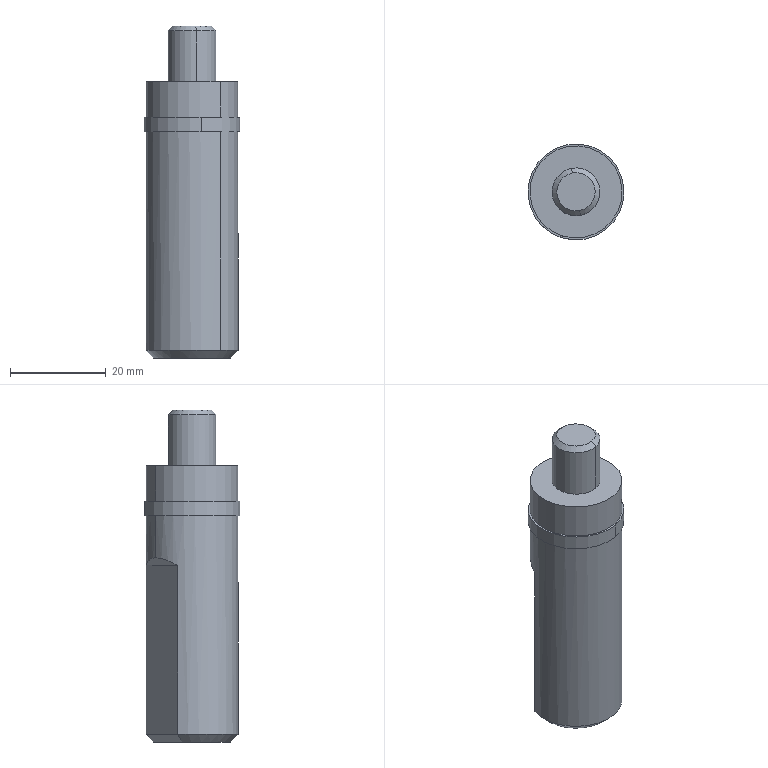Part | SolidWorks | features BaseBody 1 | 1 solid | 19 faces | box 20 x 20 x 69.2 mm | volume 17144 mm3 | cylinder 8 | plane 8 | cone 3 | commonest cylinder face diameters 19.2 x4 10 x2 20 x2
STEP:
#1=CARTESIAN_POINT('',(-577.044,-13.249,-437.6));
#2=VERTEX_POINT('',#1);
#3=CARTESIAN_POINT('',(-578.93,-3.429,-437.6));
#4=VERTEX_POINT('',#3);
#5=CARTESIAN_POINT('',(-577.987,-8.339,-437.6));
#6=DIRECTION('',(0.,0.,1.));
#7=DIRECTION('',(-1.,0.,0.));
#8=AXIS2_PLACEMENT_3D('',#5,#6,#7);
#9=CIRCLE('',#8,5.);
#10=EDGE_CURVE('',#2,#4,#9,.T.);
#11=ORIENTED_EDGE('',*,*,#10,.T.);
#12=CARTESIAN_POINT('',(-578.93,-3.429,-427.));
#13=VERTEX_POINT('',#12);
#14=CARTESIAN_POINT('',(-578.93,-3.429,-445.));
#15=DIRECTION('',(0.,0.,1.));
#16=VECTOR('',#15,1000.);
#17=LINE('',#14,#16);
#18=EDGE_CURVE('',#4,#13,#17,.T.);
#19=ORIENTED_EDGE('',*,*,#18,.T.);
#20=CARTESIAN_POINT('',(-577.044,-13.249,-427.));
#21=VERTEX_POINT('',#20);
#22=CARTESIAN_POINT('',(-577.987,-8.339,-427.));
#23=DIRECTION('',(0.,0.,-1.));
#24=DIRECTION('',(0.1886,-0.982,0.));
#25=AXIS2_PLACEMENT_3D('',#22,#23,#24);
#26=CIRCLE('',#25,5.);
#27=EDGE_CURVE('',#13,#21,#26,.T.);
#28=ORIENTED_EDGE('',*,*,#27,.T.);
#29=CARTESIAN_POINT('',(-577.044,-13.249,-445.));
#30=DIRECTION('',(0.,0.,1.));
#31=VECTOR('',#30,1000.);
#32=LINE('',#29,#31);
#33=EDGE_CURVE('',#2,#21,#32,.T.);
#34=ORIENTED_EDGE('',*,*,#33,.F.);
#35=EDGE_LOOP('',(#11,#19,#28,#34));
#36=FACE_OUTER_BOUND('',#35,.T.);
#37=CARTESIAN_POINT('',(-577.987,-8.339,-445.));
#38=DIRECTION('',(0.,0.,1.));
#39=DIRECTION('',(0.1886,-0.982,0.));
#40=AXIS2_PLACEMENT_3D('',#37,#38,#39);
#41=CYLINDRICAL_SURFACE('',#40,5.);
#42=ADVANCED_FACE('',(#36),#41,.T.);
#43=CARTESIAN_POINT('',(-577.232,-12.267,-426.));
#44=VERTEX_POINT('',#43);
#45=CARTESIAN_POINT('',(-578.741,-4.411,-426.));
#46=VERTEX_POINT('',#45);
#47=CARTESIAN_POINT('',(-577.987,-8.339,-426.));
#48=DIRECTION('',(0.,0.,1.));
#49=DIRECTION('',(0.1886,-0.982,0.));
#50=AXIS2_PLACEMENT_3D('',#47,#48,#49);
#51=CIRCLE('',#50,4.);
#52=EDGE_CURVE('',#44,#46,#51,.T.);
#53=ORIENTED_EDGE('',*,*,#52,.F.);
#54=CARTESIAN_POINT('',(-577.232,-12.267,-426.));
#55=DIRECTION('',(0.1334,-0.6944,-0.7071));
#56=VECTOR('',#55,1000.);
#57=LINE('',#54,#56);
#58=EDGE_CURVE('',#44,#21,#57,.T.);
#59=ORIENTED_EDGE('',*,*,#58,.T.);
#60=ORIENTED_EDGE('',*,*,#27,.F.);
#61=CARTESIAN_POINT('',(-578.741,-4.411,-426.));
#62=DIRECTION('',(-0.1334,0.6944,-0.7071));
#63=VECTOR('',#62,1000.);
#64=LINE('',#61,#63);
#65=EDGE_CURVE('',#46,#13,#64,.T.);
#66=ORIENTED_EDGE('',*,*,#65,.F.);
#67=EDGE_LOOP('',(#53,#59,#60,#66));
#68=FACE_OUTER_BOUND('',#67,.T.);
#69=CARTESIAN_POINT('',(-577.987,-8.339,-426.));
#70=DIRECTION('',(0.,0.,-1.));
#71=DIRECTION('',(-0.1886,0.982,0.));
#72=AXIS2_PLACEMENT_3D('',#69,#70,#71);
#73=CONICAL_SURFACE('',#72,4.,0.7854);
#74=ADVANCED_FACE('',(#68),#73,.T.);
#75=CARTESIAN_POINT('',(-572.04,-15.875,-445.));
#76=VERTEX_POINT('',#75);
#77=CARTESIAN_POINT('',(-583.933,-0.8028,-445.));
#78=VERTEX_POINT('',#77);
#79=CARTESIAN_POINT('',(-577.987,-8.339,-445.));
#80=DIRECTION('',(0.,0.,-1.));
#81=DIRECTION('',(1.,0.,0.));
#82=AXIS2_PLACEMENT_3D('',#79,#80,#81);
#83=CIRCLE('',#82,9.6);
#84=EDGE_CURVE('',#76,#78,#83,.T.);
#85=ORIENTED_EDGE('',*,*,#84,.F.);
#86=CARTESIAN_POINT('',(-572.04,-15.875,-437.6));
#87=VERTEX_POINT('',#86);
#88=CARTESIAN_POINT('',(-572.04,-15.875,-437.6));
#89=DIRECTION('',(0.,0.,1.));
#90=VECTOR('',#89,1000.);
#91=LINE('',#88,#90);
#92=EDGE_CURVE('',#76,#87,#91,.T.);
#93=ORIENTED_EDGE('',*,*,#92,.T.);
#94=CARTESIAN_POINT('',(-583.933,-0.8028,-437.6));
#95=VERTEX_POINT('',#94);
#96=CARTESIAN_POINT('',(-577.987,-8.339,-437.6));
#97=DIRECTION('',(0.,0.,1.));
#98=DIRECTION('',(0.6195,-0.785,0.));
#99=AXIS2_PLACEMENT_3D('',#96,#97,#98);
#100=CIRCLE('',#99,9.6);
#101=EDGE_CURVE('',#95,#87,#100,.T.);
#102=ORIENTED_EDGE('',*,*,#101,.F.);
#103=CARTESIAN_POINT('',(-583.933,-0.8028,-437.6));
#104=DIRECTION('',(0.,0.,1.));
#105=VECTOR('',#104,1000.);
#106=LINE('',#103,#105);
#107=EDGE_CURVE('',#78,#95,#106,.T.);
#108=ORIENTED_EDGE('',*,*,#107,.F.);
#109=EDGE_LOOP('',(#85,#93,#102,#108));
#110=FACE_OUTER_BOUND('',#109,.T.);
#111=CARTESIAN_POINT('',(-577.987,-8.339,-437.6));
#112=DIRECTION('',(0.,0.,1.));
#113=DIRECTION('',(-0.6195,0.785,0.));
#114=AXIS2_PLACEMENT_3D('',#111,#112,#113);
#115=CYLINDRICAL_SURFACE('',#114,9.6);
#116=ADVANCED_FACE('',(#110),#115,.T.);
#117=CARTESIAN_POINT('',(-579.873,1.481,-448.));
#118=VERTEX_POINT('',#117);
#119=CARTESIAN_POINT('',(-576.1,-18.16,-448.));
#120=VERTEX_POINT('',#119);
#121=CARTESIAN_POINT('',(-577.987,-8.339,-448.));
#122=DIRECTION('',(0.,0.,-1.));
#123=DIRECTION('',(-0.1886,0.982,0.));
#124=AXIS2_PLACEMENT_3D('',#121,#122,#123);
#125=CIRCLE('',#124,10.);
#126=EDGE_CURVE('',#118,#120,#125,.T.);
#127=ORIENTED_EDGE('',*,*,#126,.F.);
#128=CARTESIAN_POINT('',(-579.873,1.481,-445.));
#129=VERTEX_POINT('',#128);
#130=CARTESIAN_POINT('',(-579.873,1.481,-448.));
#131=DIRECTION('',(0.,0.,1.));
#132=VECTOR('',#131,1000.);
#133=LINE('',#130,#132);
#134=EDGE_CURVE('',#118,#129,#133,.T.);
#135=ORIENTED_EDGE('',*,*,#134,.T.);
#136=CARTESIAN_POINT('',(-576.1,-18.16,-445.));
#137=VERTEX_POINT('',#136);
#138=CARTESIAN_POINT('',(-577.987,-8.339,-445.));
#139=DIRECTION('',(0.,0.,-1.));
#140=DIRECTION('',(-0.1886,0.982,0.));
#141=AXIS2_PLACEMENT_3D('',#138,#139,#140);
#142=CIRCLE('',#141,10.);
#143=EDGE_CURVE('',#129,#137,#142,.T.);
#144=ORIENTED_EDGE('',*,*,#143,.T.);
#145=CARTESIAN_POINT('',(-576.1,-18.16,-448.));
#146=DIRECTION('',(0.,0.,1.));
#147=VECTOR('',#146,1000.);
#148=LINE('',#145,#147);
#149=EDGE_CURVE('',#120,#137,#148,.T.);
#150=ORIENTED_EDGE('',*,*,#149,.F.);
#151=EDGE_LOOP('',(#127,#135,#144,#150));
#152=FACE_OUTER_BOUND('',#151,.T.);
#153=CARTESIAN_POINT('',(-577.987,-8.339,-448.));
#154=DIRECTION('',(0.,0.,1.));
#155=DIRECTION('',(0.1886,-0.982,0.));
#156=AXIS2_PLACEMENT_3D('',#153,#154,#155);
#157=CYLINDRICAL_SURFACE('',#156,10.);
#158=ADVANCED_FACE('',(#152),#157,.T.);
#159=CARTESIAN_POINT('',(-587.108,-5.346,-493.6));
#160=VERTEX_POINT('',#159);
#161=CARTESIAN_POINT('',(-572.04,-15.875,-493.6));
#162=VERTEX_POINT('',#161);
#163=CARTESIAN_POINT('',(-577.987,-8.339,-493.6));
#164=DIRECTION('',(0.,0.,1.));
#165=DIRECTION('',(0.6195,-0.785,0.));
#166=AXIS2_PLACEMENT_3D('',#163,#164,#165);
#167=CIRCLE('',#166,9.6);
#168=EDGE_CURVE('',#160,#162,#167,.T.);
#169=ORIENTED_EDGE('',*,*,#168,.T.);
#170=CARTESIAN_POINT('',(-572.04,-15.875,-448.));
#171=VERTEX_POINT('',#170);
#172=CARTESIAN_POINT('',(-572.04,-15.875,-437.6));
#173=DIRECTION('',(0.,0.,1.));
#174=VECTOR('',#173,1000.);
#175=LINE('',#172,#174);
#176=EDGE_CURVE('',#162,#171,#175,.T.);
#177=ORIENTED_EDGE('',*,*,#176,.T.);
#178=CARTESIAN_POINT('',(-583.933,-0.8028,-448.));
#179=VERTEX_POINT('',#178);
#180=CARTESIAN_POINT('',(-577.987,-8.339,-448.));
#181=DIRECTION('',(0.,0.,-1.));
#182=DIRECTION('',(1.,0.,0.));
#183=AXIS2_PLACEMENT_3D('',#180,#181,#182);
#184=CIRCLE('',#183,9.6);
#185=EDGE_CURVE('',#171,#179,#184,.T.);
#186=ORIENTED_EDGE('',*,*,#185,.T.);
#187=CARTESIAN_POINT('',(-583.933,-0.8028,-456.8));
#188=VERTEX_POINT('',#187);
#189=CARTESIAN_POINT('',(-583.933,-0.8028,-437.6));
#190=DIRECTION('',(0.,0.,1.));
#191=VECTOR('',#190,1000.);
#192=LINE('',#189,#191);
#193=EDGE_CURVE('',#188,#179,#192,.T.);
#194=ORIENTED_EDGE('',*,*,#193,.F.);
#195=CARTESIAN_POINT('',(-587.108,-5.346,-458.4));
#196=VERTEX_POINT('',#195);
#197=CARTESIAN_POINT('',(-583.933,-0.8028,-456.8));
#198=CARTESIAN_POINT('',(-585.426,-1.981,-456.8));
#199=CARTESIAN_POINT('',(-586.515,-3.539,-457.349));
#200=CARTESIAN_POINT('',(-587.108,-5.346,-458.4));
#201=(BOUNDED_CURVE()B_SPLINE_CURVE(3,(#197,#198,#199,#200),.UNSPECIFIED.,.F.,.F.)B_SPLINE_CURVE_WITH_KNOTS((4,4),(0.,0.5857),.UNSPECIFIED.)CURVE()GEOMETRIC_REPRESENTATION_ITEM()RATIONAL_B_SPLINE_CURVE((1.,0.9716,0.9716,1.))REPRESENTATION_ITEM(''));
#202=EDGE_CURVE('',#188,#196,#201,.T.);
#203=ORIENTED_EDGE('',*,*,#202,.T.);
#204=CARTESIAN_POINT('',(-587.108,-5.346,-456.8));
#205=DIRECTION('',(0.,0.,1.));
#206=VECTOR('',#205,1000.);
#207=LINE('',#204,#206);
#208=EDGE_CURVE('',#160,#196,#207,.T.);
#209=ORIENTED_EDGE('',*,*,#208,.F.);
#210=EDGE_LOOP('',(#169,#177,#186,#194,#203,#209));
#211=FACE_OUTER_BOUND('',#210,.T.);
#212=CARTESIAN_POINT('',(-577.987,-8.339,-437.6));
#213=DIRECTION('',(0.,0.,1.));
#214=DIRECTION('',(-0.6195,0.785,0.));
#215=AXIS2_PLACEMENT_3D('',#212,#213,#214);
#216=CYLINDRICAL_SURFACE('',#215,9.6);
#217=ADVANCED_FACE('',(#211),#216,.T.);
#218=ORIENTED_EDGE('',*,*,#176,.F.);
#219=CARTESIAN_POINT('',(-578.777,1.228,-493.6));
#220=VERTEX_POINT('',#219);
#221=CARTESIAN_POINT('',(-577.987,-8.339,-493.6));
#222=DIRECTION('',(0.,0.,1.));
#223=DIRECTION('',(0.6195,-0.785,0.));
#224=AXIS2_PLACEMENT_3D('',#221,#222,#223);
#225=CIRCLE('',#224,9.6);
#226=EDGE_CURVE('',#162,#220,#225,.T.);
#227=ORIENTED_EDGE('',*,*,#226,.T.);
#228=CARTESIAN_POINT('',(-578.777,1.228,-458.4));
#229=VERTEX_POINT('',#228);
#230=CARTESIAN_POINT('',(-578.777,1.228,-456.8));
#231=DIRECTION('',(0.,0.,1.));
#232=VECTOR('',#231,1000.);
#233=LINE('',#230,#232);
#234=EDGE_CURVE('',#220,#229,#233,.T.);
#235=ORIENTED_EDGE('',*,*,#234,.T.);
#236=CARTESIAN_POINT('',(-578.777,1.228,-458.4));
#237=CARTESIAN_POINT('',(-580.672,1.072,-457.349));
#238=CARTESIAN_POINT('',(-582.441,0.3751,-456.8));
#239=CARTESIAN_POINT('',(-583.933,-0.8028,-456.8));
#240=(BOUNDED_CURVE()B_SPLINE_CURVE(3,(#236,#237,#238,#239),.UNSPECIFIED.,.F.,.F.)B_SPLINE_CURVE_WITH_KNOTS((4,4),(5.697,6.283),.UNSPECIFIED.)CURVE()GEOMETRIC_REPRESENTATION_ITEM()RATIONAL_B_SPLINE_CURVE((1.,0.9716,0.9716,1.))REPRESENTATION_ITEM(''));
#241=EDGE_CURVE('',#229,#188,#240,.T.);
#242=ORIENTED_EDGE('',*,*,#241,.T.);
#243=ORIENTED_EDGE('',*,*,#193,.T.);
#244=CARTESIAN_POINT('',(-577.987,-8.339,-448.));
#245=DIRECTION('',(0.,0.,-1.));
#246=DIRECTION('',(1.,0.,0.));
#247=AXIS2_PLACEMENT_3D('',#244,#245,#246);
#248=CIRCLE('',#247,9.6);
#249=EDGE_CURVE('',#179,#171,#248,.T.);
#250=ORIENTED_EDGE('',*,*,#249,.T.);
#251=EDGE_LOOP('',(#218,#227,#235,#242,#243,#250));
#252=FACE_OUTER_BOUND('',#251,.T.);
#253=CARTESIAN_POINT('',(-577.987,-8.339,-437.6));
#254=DIRECTION('',(0.,0.,1.));
#255=DIRECTION('',(-0.6195,0.785,0.));
#256=AXIS2_PLACEMENT_3D('',#253,#254,#255);
#257=CYLINDRICAL_SURFACE('',#256,9.6);
#258=ADVANCED_FACE('',(#252),#257,.T.);
#259=CARTESIAN_POINT('',(-585.719,-6.288,-495.2));
#260=VERTEX_POINT('',#259);
#261=CARTESIAN_POINT('',(-578.183,-0.3415,-495.2));
#262=VERTEX_POINT('',#261);
#263=CARTESIAN_POINT('',(-586.117,-6.602,-495.2));
#264=DIRECTION('',(0.785,0.6195,0.));
#265=VECTOR('',#264,1000.);
#266=LINE('',#263,#265);
#267=EDGE_CURVE('',#260,#262,#266,.T.);
#268=ORIENTED_EDGE('',*,*,#267,.T.);
#269=CARTESIAN_POINT('',(-577.987,-8.339,-495.2));
#270=DIRECTION('',(0.,0.,-1.));
#271=DIRECTION('',(0.6195,-0.785,0.));
#272=AXIS2_PLACEMENT_3D('',#269,#270,#271);
#273=CIRCLE('',#272,8.);
#274=EDGE_CURVE('',#262,#260,#273,.T.);
#275=ORIENTED_EDGE('',*,*,#274,.T.);
#276=EDGE_LOOP('',(#268,#275));
#277=FACE_OUTER_BOUND('',#276,.T.);
#278=CARTESIAN_POINT('',(-577.987,-8.339,-495.2));
#279=DIRECTION('',(0.,0.,-1.));
#280=DIRECTION('',(0.6195,-0.785,0.));
#281=AXIS2_PLACEMENT_3D('',#278,#279,#280);
#282=PLANE('',#281);
#283=ADVANCED_FACE('',(#277),#282,.T.);
#284=ORIENTED_EDGE('',*,*,#208,.T.);
#285=CARTESIAN_POINT('',(-587.108,-5.346,-458.4));
#286=DIRECTION('',(0.785,0.6195,0.));
#287=VECTOR('',#286,1000.);
#288=LINE('',#285,#287);
#289=EDGE_CURVE('',#196,#229,#288,.T.);
#290=ORIENTED_EDGE('',*,*,#289,.T.);
#291=ORIENTED_EDGE('',*,*,#234,.F.);
#292=CARTESIAN_POINT('',(-578.777,1.228,-493.6));
#293=DIRECTION('',(-0.785,-0.6195,0.));
#294=VECTOR('',#293,1000.);
#295=LINE('',#292,#294);
#296=EDGE_CURVE('',#220,#160,#295,.T.);
#297=ORIENTED_EDGE('',*,*,#296,.T.);
#298=EDGE_LOOP('',(#284,#290,#291,#297));
#299=FACE_OUTER_BOUND('',#298,.T.);
#300=CARTESIAN_POINT('',(-587.108,-5.346,-456.8));
#301=DIRECTION('',(0.6195,-0.785,0.));
#302=DIRECTION('',(0.785,0.6195,0.));
#303=AXIS2_PLACEMENT_3D('',#300,#301,#302);
#304=PLANE('',#303);
#305=ADVANCED_FACE('',(#299),#304,.F.);
#306=CARTESIAN_POINT('',(-578.183,-0.3415,-495.2));
#307=CARTESIAN_POINT('',(-578.373,0.186,-494.668));
#308=CARTESIAN_POINT('',(-578.572,0.7089,-494.135));
#309=CARTESIAN_POINT('',(-578.777,1.228,-493.6));
#310=B_SPLINE_CURVE_WITH_KNOTS('',3,(#306,#307,#308,#309),.UNSPECIFIED.,.F.,.F.,(4,4),(0.,0.002319),.UNSPECIFIED.);
#311=EDGE_CURVE('',#262,#220,#310,.T.);
#312=ORIENTED_EDGE('',*,*,#311,.F.);
#313=ORIENTED_EDGE('',*,*,#267,.F.);
#314=CARTESIAN_POINT('',(-587.108,-5.346,-493.6));
#315=CARTESIAN_POINT('',(-586.651,-5.666,-494.135));
#316=CARTESIAN_POINT('',(-586.188,-5.98,-494.668));
#317=CARTESIAN_POINT('',(-585.719,-6.288,-495.2));
#318=B_SPLINE_CURVE_WITH_KNOTS('',3,(#314,#315,#316,#317),.UNSPECIFIED.,.F.,.F.,(4,4),(0.,0.002319),.UNSPECIFIED.);
#319=EDGE_CURVE('',#160,#260,#318,.T.);
#320=ORIENTED_EDGE('',*,*,#319,.F.);
#321=ORIENTED_EDGE('',*,*,#296,.F.);
#322=EDGE_LOOP('',(#312,#313,#320,#321));
#323=FACE_OUTER_BOUND('',#322,.T.);
#324=CARTESIAN_POINT('',(-587.108,-5.346,-493.6));
#325=DIRECTION('',(-0.438,0.5551,-0.7071));
#326=DIRECTION('',(-0.785,-0.6195,0.));
#327=AXIS2_PLACEMENT_3D('',#324,#325,#326);
#328=PLANE('',#327);
#329=ADVANCED_FACE('',(#323),#328,.T.);
#330=ORIENTED_EDGE('',*,*,#319,.T.);
#331=ORIENTED_EDGE('',*,*,#274,.F.);
#332=ORIENTED_EDGE('',*,*,#311,.T.);
#333=ORIENTED_EDGE('',*,*,#226,.F.);
#334=ORIENTED_EDGE('',*,*,#168,.F.);
#335=EDGE_LOOP('',(#330,#331,#332,#333,#334));
#336=FACE_OUTER_BOUND('',#335,.T.);
#337=CARTESIAN_POINT('',(-577.987,-8.339,-495.2));
#338=DIRECTION('',(0.,0.,1.));
#339=DIRECTION('',(-0.6195,0.785,0.));
#340=AXIS2_PLACEMENT_3D('',#337,#338,#339);
#341=CONICAL_SURFACE('',#340,8.,0.7854);
#342=ADVANCED_FACE('',(#336),#341,.T.);
#343=ORIENTED_EDGE('',*,*,#289,.F.);
#344=ORIENTED_EDGE('',*,*,#202,.F.);
#345=ORIENTED_EDGE('',*,*,#241,.F.);
#346=EDGE_LOOP('',(#343,#344,#345));
#347=FACE_OUTER_BOUND('',#346,.T.);
#348=CARTESIAN_POINT('',(-583.933,-0.8028,-456.8));
#349=DIRECTION('',(0.438,-0.5551,0.7071));
#350=DIRECTION('',(0.785,0.6195,0.));
#351=AXIS2_PLACEMENT_3D('',#348,#349,#350);
#352=PLANE('',#351);
#353=ADVANCED_FACE('',(#347),#352,.F.);
#354=CARTESIAN_POINT('',(-577.987,-8.339,-448.));
#355=DIRECTION('',(0.,0.,-1.));
#356=DIRECTION('',(-0.1886,0.982,0.));
#357=AXIS2_PLACEMENT_3D('',#354,#355,#356);
#358=CIRCLE('',#357,10.);
#359=EDGE_CURVE('',#120,#118,#358,.T.);
#360=ORIENTED_EDGE('',*,*,#359,.T.);
#361=ORIENTED_EDGE('',*,*,#126,.T.);
#362=EDGE_LOOP('',(#360,#361));
#363=FACE_OUTER_BOUND('',#362,.T.);
#364=ORIENTED_EDGE('',*,*,#249,.F.);
#365=ORIENTED_EDGE('',*,*,#185,.F.);
#366=EDGE_LOOP('',(#364,#365));
#367=FACE_BOUND('',#366,.T.);
#368=CARTESIAN_POINT('',(-577.987,-8.339,-448.));
#369=DIRECTION('',(0.,0.,-1.));
#370=DIRECTION('',(-0.1886,0.982,0.));
#371=AXIS2_PLACEMENT_3D('',#368,#369,#370);
#372=PLANE('',#371);
#373=ADVANCED_FACE('',(#363,#367),#372,.T.);
#374=CARTESIAN_POINT('',(-577.987,-8.339,-445.));
#375=DIRECTION('',(0.,0.,-1.));
#376=DIRECTION('',(-0.1886,0.982,0.));
#377=AXIS2_PLACEMENT_3D('',#374,#375,#376);
#378=CIRCLE('',#377,10.);
#379=EDGE_CURVE('',#137,#129,#378,.T.);
#380=ORIENTED_EDGE('',*,*,#379,.F.);
#381=ORIENTED_EDGE('',*,*,#143,.F.);
#382=EDGE_LOOP('',(#380,#381));
#383=FACE_OUTER_BOUND('',#382,.T.);
#384=CARTESIAN_POINT('',(-577.987,-8.339,-445.));
#385=DIRECTION('',(0.,0.,-1.));
#386=DIRECTION('',(1.,0.,0.));
#387=AXIS2_PLACEMENT_3D('',#384,#385,#386);
#388=CIRCLE('',#387,9.6);
#389=EDGE_CURVE('',#78,#76,#388,.T.);
#390=ORIENTED_EDGE('',*,*,#389,.T.);
#391=ORIENTED_EDGE('',*,*,#84,.T.);
#392=EDGE_LOOP('',(#390,#391));
#393=FACE_BOUND('',#392,.T.);
#394=CARTESIAN_POINT('',(-577.987,-8.339,-445.));
#395=DIRECTION('',(0.,0.,-1.));
#396=DIRECTION('',(-0.1886,0.982,0.));
#397=AXIS2_PLACEMENT_3D('',#394,#395,#396);
#398=PLANE('',#397);
#399=ADVANCED_FACE('',(#383,#393),#398,.F.);
#400=ORIENTED_EDGE('',*,*,#134,.F.);
#401=ORIENTED_EDGE('',*,*,#359,.F.);
#402=ORIENTED_EDGE('',*,*,#149,.T.);
#403=ORIENTED_EDGE('',*,*,#379,.T.);
#404=EDGE_LOOP('',(#400,#401,#402,#403));
#405=FACE_OUTER_BOUND('',#404,.T.);
#406=CARTESIAN_POINT('',(-577.987,-8.339,-448.));
#407=DIRECTION('',(0.,0.,1.));
#408=DIRECTION('',(0.1886,-0.982,0.));
#409=AXIS2_PLACEMENT_3D('',#406,#407,#408);
#410=CYLINDRICAL_SURFACE('',#409,10.);
#411=ADVANCED_FACE('',(#405),#410,.T.);
#412=ORIENTED_EDGE('',*,*,#10,.F.);
#413=CARTESIAN_POINT('',(-577.987,-8.339,-437.6));
#414=DIRECTION('',(0.,0.,1.));
#415=DIRECTION('',(-1.,0.,0.));
#416=AXIS2_PLACEMENT_3D('',#413,#414,#415);
#417=CIRCLE('',#416,5.);
#418=EDGE_CURVE('',#4,#2,#417,.T.);
#419=ORIENTED_EDGE('',*,*,#418,.F.);
#420=EDGE_LOOP('',(#412,#419));
#421=FACE_BOUND('',#420,.T.);
#422=ORIENTED_EDGE('',*,*,#101,.T.);
#423=CARTESIAN_POINT('',(-577.987,-8.339,-437.6));
#424=DIRECTION('',(0.,0.,1.));
#425=DIRECTION('',(0.6195,-0.785,0.));
#426=AXIS2_PLACEMENT_3D('',#423,#424,#425);
#427=CIRCLE('',#426,9.6);
#428=EDGE_CURVE('',#87,#95,#427,.T.);
#429=ORIENTED_EDGE('',*,*,#428,.T.);
#430=EDGE_LOOP('',(#422,#429));
#431=FACE_OUTER_BOUND('',#430,.T.);
#432=CARTESIAN_POINT('',(-584.663,0.1218,-437.6));
#433=DIRECTION('',(0.,0.,1.));
#434=DIRECTION('',(-1.,0.,0.));
#435=AXIS2_PLACEMENT_3D('',#432,#433,#434);
#436=PLANE('',#435);
#437=ADVANCED_FACE('',(#421,#431),#436,.T.);
#438=ORIENTED_EDGE('',*,*,#92,.F.);
#439=ORIENTED_EDGE('',*,*,#389,.F.);
#440=ORIENTED_EDGE('',*,*,#107,.T.);
#441=ORIENTED_EDGE('',*,*,#428,.F.);
#442=EDGE_LOOP('',(#438,#439,#440,#441));
#443=FACE_OUTER_BOUND('',#442,.T.);
#444=CARTESIAN_POINT('',(-577.987,-8.339,-437.6));
#445=DIRECTION('',(0.,0.,1.));
#446=DIRECTION('',(-0.6195,0.785,0.));
#447=AXIS2_PLACEMENT_3D('',#444,#445,#446);
#448=CYLINDRICAL_SURFACE('',#447,9.6);
#449=ADVANCED_FACE('',(#443),#448,.T.);
#450=CARTESIAN_POINT('',(-577.987,-8.339,-426.));
#451=DIRECTION('',(0.,0.,1.));
#452=DIRECTION('',(0.1886,-0.982,0.));
#453=AXIS2_PLACEMENT_3D('',#450,#451,#452);
#454=CIRCLE('',#453,4.);
#455=EDGE_CURVE('',#46,#44,#454,.T.);
#456=ORIENTED_EDGE('',*,*,#455,.T.);
#457=ORIENTED_EDGE('',*,*,#52,.T.);
#458=EDGE_LOOP('',(#456,#457));
#459=FACE_OUTER_BOUND('',#458,.T.);
#460=CARTESIAN_POINT('',(-577.987,-8.339,-426.));
#461=DIRECTION('',(0.,0.,1.));
#462=DIRECTION('',(0.1886,-0.982,0.));
#463=AXIS2_PLACEMENT_3D('',#460,#461,#462);
#464=PLANE('',#463);
#465=ADVANCED_FACE('',(#459),#464,.T.);
#466=ORIENTED_EDGE('',*,*,#58,.F.);
#467=ORIENTED_EDGE('',*,*,#455,.F.);
#468=ORIENTED_EDGE('',*,*,#65,.T.);
#469=CARTESIAN_POINT('',(-577.987,-8.339,-427.));
#470=DIRECTION('',(0.,0.,-1.));
#471=DIRECTION('',(0.1886,-0.982,0.));
#472=AXIS2_PLACEMENT_3D('',#469,#470,#471);
#473=CIRCLE('',#472,5.);
#474=EDGE_CURVE('',#21,#13,#473,.T.);
#475=ORIENTED_EDGE('',*,*,#474,.F.);
#476=EDGE_LOOP('',(#466,#467,#468,#475));
#477=FACE_OUTER_BOUND('',#476,.T.);
#478=CARTESIAN_POINT('',(-577.987,-8.339,-426.));
#479=DIRECTION('',(0.,0.,-1.));
#480=DIRECTION('',(-0.1886,0.982,0.));
#481=AXIS2_PLACEMENT_3D('',#478,#479,#480);
#482=CONICAL_SURFACE('',#481,4.,0.7854);
#483=ADVANCED_FACE('',(#477),#482,.T.);
#484=ORIENTED_EDGE('',*,*,#18,.F.);
#485=ORIENTED_EDGE('',*,*,#418,.T.);
#486=ORIENTED_EDGE('',*,*,#33,.T.);
#487=ORIENTED_EDGE('',*,*,#474,.T.);
#488=EDGE_LOOP('',(#484,#485,#486,#487));
#489=FACE_OUTER_BOUND('',#488,.T.);
#490=CARTESIAN_POINT('',(-577.987,-8.339,-445.));
#491=DIRECTION('',(0.,0.,1.));
#492=DIRECTION('',(0.1886,-0.982,0.));
#493=AXIS2_PLACEMENT_3D('',#490,#491,#492);
#494=CYLINDRICAL_SURFACE('',#493,5.);
#495=ADVANCED_FACE('',(#489),#494,.T.);
#496=CLOSED_SHELL('',(#42,#74,#116,#158,#217,#258,#283,#305,#329,#342,#353,#373,#399,#411,#437,#449,#465,#483,#495));
#497=MANIFOLD_SOLID_BREP('',#496);
#498=CARTESIAN_POINT('',(0.,0.,0.));
#499=DIRECTION('',(0.,0.,1.));
#500=DIRECTION('',(1.,0.,0.));
#501=AXIS2_PLACEMENT_3D('',#498,#499,#500);
#502=(LENGTH_UNIT()NAMED_UNIT(*)SI_UNIT(.MILLI.,.METRE.));
#503=UNCERTAINTY_MEASURE_WITH_UNIT(LENGTH_MEASURE(0.00001),#502,'','');
#504=(NAMED_UNIT(*)PLANE_ANGLE_UNIT()SI_UNIT($,.RADIAN.));
#505=(NAMED_UNIT(*)SI_UNIT($,.STERADIAN.)SOLID_ANGLE_UNIT());
#506=(GEOMETRIC_REPRESENTATION_CONTEXT(3)GLOBAL_UNCERTAINTY_ASSIGNED_CONTEXT((#503))GLOBAL_UNIT_ASSIGNED_CONTEXT((#502,#504,#505))REPRESENTATION_CONTEXT('',''));
#507=ADVANCED_BREP_SHAPE_REPRESENTATION('',(#497,#501),#506);